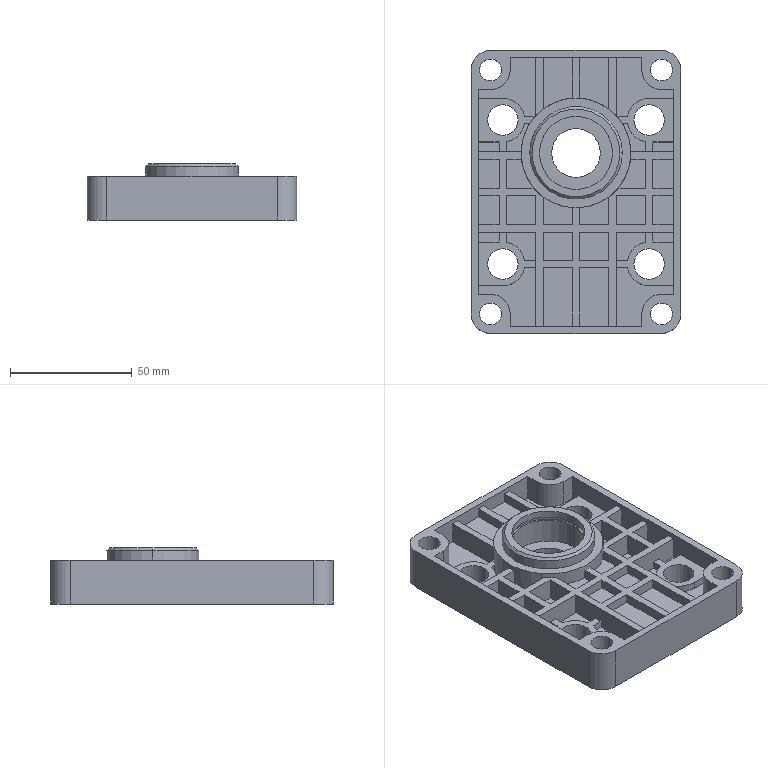Part | SolidWorks | features ICE 11, BossThin 2, Chamfer 1, Extrusion 1, HoleWzd 1, MirrorPattern 1, MoveFace 1, Split 1 | 1 solid | 195 faces | box 86 x 116 x 23 mm | volume 111724 mm3 | plane 141 | cylinder 48 | cone 6 | commonest cylinder face diameters 9 x8 12.5 x8 16 x8 18 x8 8 x4 30 x4